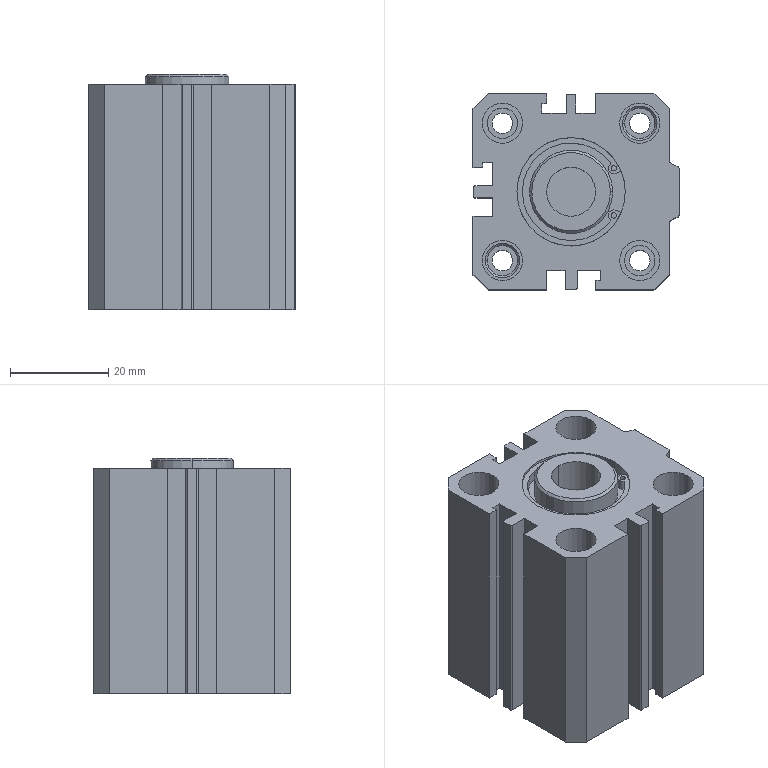Part | SolidWorks | features BaseBody 1 | 1 solid | 207 faces | box 42 x 40 x 48 mm | volume 48635 mm3 | cylinder 116 | plane 75 | cone 10 | spline 6 | commonest cylinder face diameters 5 x50 6.2 x16 8.2 x16 0.6 x8 4.2 x8 1.105 x4